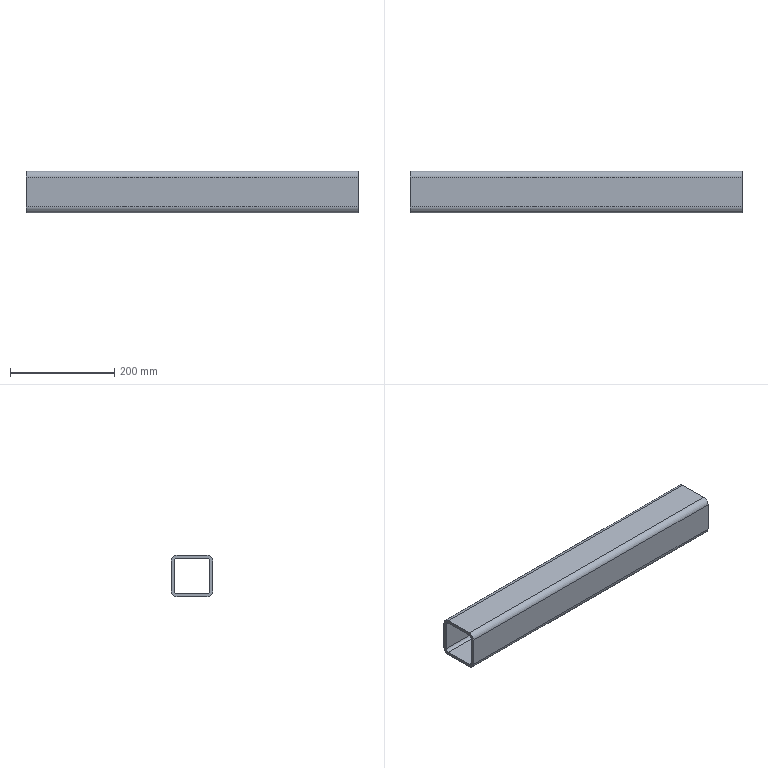Part | SolidWorks | features Extrusion 1 | 1 solid | 18 faces | box 638 x 80 x 80 mm | volume 1029649 mm3 | plane 10 | cylinder 8 | commonest cylinder face diameters 11.429 x4 22.857 x4
STEP:
#1=CARTESIAN_POINT('',(249.,-40.,-28.571));
#2=VERTEX_POINT('',#1);
#3=CARTESIAN_POINT('',(249.,-28.571,-40.));
#4=VERTEX_POINT('',#3);
#5=CARTESIAN_POINT('',(249.,-28.571,-28.571));
#6=DIRECTION('',(1.,0.,0.));
#7=DIRECTION('',(0.,0.,-1.));
#8=AXIS2_PLACEMENT_3D('',#5,#6,#7);
#9=CIRCLE('',#8,11.429);
#10=EDGE_CURVE('',#2,#4,#9,.T.);
#11=ORIENTED_EDGE('',*,*,#10,.F.);
#12=CARTESIAN_POINT('',(-389.,-40.,-28.571));
#13=VERTEX_POINT('',#12);
#14=CARTESIAN_POINT('',(-389.,-40.,-28.571));
#15=DIRECTION('',(1.,0.,0.));
#16=VECTOR('',#15,1000.);
#17=LINE('',#14,#16);
#18=EDGE_CURVE('',#13,#2,#17,.T.);
#19=ORIENTED_EDGE('',*,*,#18,.F.);
#20=CARTESIAN_POINT('',(-389.,-28.571,-40.));
#21=VERTEX_POINT('',#20);
#22=CARTESIAN_POINT('',(-389.,-28.571,-28.571));
#23=DIRECTION('',(1.,0.,0.));
#24=DIRECTION('',(0.,0.,-1.));
#25=AXIS2_PLACEMENT_3D('',#22,#23,#24);
#26=CIRCLE('',#25,11.429);
#27=EDGE_CURVE('',#13,#21,#26,.T.);
#28=ORIENTED_EDGE('',*,*,#27,.T.);
#29=CARTESIAN_POINT('',(-389.,-28.571,-40.));
#30=DIRECTION('',(1.,0.,0.));
#31=VECTOR('',#30,1000.);
#32=LINE('',#29,#31);
#33=EDGE_CURVE('',#21,#4,#32,.T.);
#34=ORIENTED_EDGE('',*,*,#33,.T.);
#35=EDGE_LOOP('',(#11,#19,#28,#34));
#36=FACE_OUTER_BOUND('',#35,.T.);
#37=CARTESIAN_POINT('',(-389.,-28.571,-28.571));
#38=DIRECTION('',(1.,0.,0.));
#39=DIRECTION('',(0.,0.,-1.));
#40=AXIS2_PLACEMENT_3D('',#37,#38,#39);
#41=CYLINDRICAL_SURFACE('',#40,11.429);
#42=ADVANCED_FACE('',(#36),#41,.T.);
#43=CARTESIAN_POINT('',(249.,-40.,28.571));
#44=VERTEX_POINT('',#43);
#45=CARTESIAN_POINT('',(249.,-40.,28.571));
#46=DIRECTION('',(0.,0.,-1.));
#47=VECTOR('',#46,1000.);
#48=LINE('',#45,#47);
#49=EDGE_CURVE('',#44,#2,#48,.T.);
#50=ORIENTED_EDGE('',*,*,#49,.F.);
#51=CARTESIAN_POINT('',(-389.,-40.,28.571));
#52=VERTEX_POINT('',#51);
#53=CARTESIAN_POINT('',(-389.,-40.,28.571));
#54=DIRECTION('',(1.,0.,0.));
#55=VECTOR('',#54,1000.);
#56=LINE('',#53,#55);
#57=EDGE_CURVE('',#52,#44,#56,.T.);
#58=ORIENTED_EDGE('',*,*,#57,.F.);
#59=CARTESIAN_POINT('',(-389.,-40.,28.571));
#60=DIRECTION('',(0.,0.,-1.));
#61=VECTOR('',#60,1000.);
#62=LINE('',#59,#61);
#63=EDGE_CURVE('',#52,#13,#62,.T.);
#64=ORIENTED_EDGE('',*,*,#63,.T.);
#65=ORIENTED_EDGE('',*,*,#18,.T.);
#66=EDGE_LOOP('',(#50,#58,#64,#65));
#67=FACE_OUTER_BOUND('',#66,.T.);
#68=CARTESIAN_POINT('',(-389.,-40.,28.571));
#69=DIRECTION('',(0.,-1.,0.));
#70=DIRECTION('',(0.,0.,-1.));
#71=AXIS2_PLACEMENT_3D('',#68,#69,#70);
#72=PLANE('',#71);
#73=ADVANCED_FACE('',(#67),#72,.T.);
#74=CARTESIAN_POINT('',(249.,-28.571,40.));
#75=VERTEX_POINT('',#74);
#76=CARTESIAN_POINT('',(249.,-28.571,28.571));
#77=DIRECTION('',(1.,0.,0.));
#78=DIRECTION('',(0.,0.,-1.));
#79=AXIS2_PLACEMENT_3D('',#76,#77,#78);
#80=CIRCLE('',#79,11.429);
#81=EDGE_CURVE('',#75,#44,#80,.T.);
#82=ORIENTED_EDGE('',*,*,#81,.F.);
#83=CARTESIAN_POINT('',(-389.,-28.571,40.));
#84=VERTEX_POINT('',#83);
#85=CARTESIAN_POINT('',(-389.,-28.571,40.));
#86=DIRECTION('',(1.,0.,0.));
#87=VECTOR('',#86,1000.);
#88=LINE('',#85,#87);
#89=EDGE_CURVE('',#84,#75,#88,.T.);
#90=ORIENTED_EDGE('',*,*,#89,.F.);
#91=CARTESIAN_POINT('',(-389.,-28.571,28.571));
#92=DIRECTION('',(1.,0.,0.));
#93=DIRECTION('',(0.,0.,-1.));
#94=AXIS2_PLACEMENT_3D('',#91,#92,#93);
#95=CIRCLE('',#94,11.429);
#96=EDGE_CURVE('',#84,#52,#95,.T.);
#97=ORIENTED_EDGE('',*,*,#96,.T.);
#98=ORIENTED_EDGE('',*,*,#57,.T.);
#99=EDGE_LOOP('',(#82,#90,#97,#98));
#100=FACE_OUTER_BOUND('',#99,.T.);
#101=CARTESIAN_POINT('',(-389.,-28.571,28.571));
#102=DIRECTION('',(1.,0.,0.));
#103=DIRECTION('',(0.,0.,-1.));
#104=AXIS2_PLACEMENT_3D('',#101,#102,#103);
#105=CYLINDRICAL_SURFACE('',#104,11.429);
#106=ADVANCED_FACE('',(#100),#105,.T.);
#107=CARTESIAN_POINT('',(249.,28.571,40.));
#108=VERTEX_POINT('',#107);
#109=CARTESIAN_POINT('',(249.,28.571,40.));
#110=DIRECTION('',(0.,-1.,0.));
#111=VECTOR('',#110,1000.);
#112=LINE('',#109,#111);
#113=EDGE_CURVE('',#108,#75,#112,.T.);
#114=ORIENTED_EDGE('',*,*,#113,.F.);
#115=CARTESIAN_POINT('',(-389.,28.571,40.));
#116=VERTEX_POINT('',#115);
#117=CARTESIAN_POINT('',(-389.,28.571,40.));
#118=DIRECTION('',(1.,0.,0.));
#119=VECTOR('',#118,1000.);
#120=LINE('',#117,#119);
#121=EDGE_CURVE('',#116,#108,#120,.T.);
#122=ORIENTED_EDGE('',*,*,#121,.F.);
#123=CARTESIAN_POINT('',(-389.,28.571,40.));
#124=DIRECTION('',(0.,-1.,0.));
#125=VECTOR('',#124,1000.);
#126=LINE('',#123,#125);
#127=EDGE_CURVE('',#116,#84,#126,.T.);
#128=ORIENTED_EDGE('',*,*,#127,.T.);
#129=ORIENTED_EDGE('',*,*,#89,.T.);
#130=EDGE_LOOP('',(#114,#122,#128,#129));
#131=FACE_OUTER_BOUND('',#130,.T.);
#132=CARTESIAN_POINT('',(-389.,28.571,40.));
#133=DIRECTION('',(0.,0.,1.));
#134=DIRECTION('',(1.,0.,0.));
#135=AXIS2_PLACEMENT_3D('',#132,#133,#134);
#136=PLANE('',#135);
#137=ADVANCED_FACE('',(#131),#136,.T.);
#138=CARTESIAN_POINT('',(249.,40.,28.571));
#139=VERTEX_POINT('',#138);
#140=CARTESIAN_POINT('',(249.,28.571,28.571));
#141=DIRECTION('',(1.,0.,0.));
#142=DIRECTION('',(0.,0.,-1.));
#143=AXIS2_PLACEMENT_3D('',#140,#141,#142);
#144=CIRCLE('',#143,11.429);
#145=EDGE_CURVE('',#139,#108,#144,.T.);
#146=ORIENTED_EDGE('',*,*,#145,.F.);
#147=CARTESIAN_POINT('',(-389.,40.,28.571));
#148=VERTEX_POINT('',#147);
#149=CARTESIAN_POINT('',(-389.,40.,28.571));
#150=DIRECTION('',(1.,0.,0.));
#151=VECTOR('',#150,1000.);
#152=LINE('',#149,#151);
#153=EDGE_CURVE('',#148,#139,#152,.T.);
#154=ORIENTED_EDGE('',*,*,#153,.F.);
#155=CARTESIAN_POINT('',(-389.,28.571,28.571));
#156=DIRECTION('',(1.,0.,0.));
#157=DIRECTION('',(0.,0.,-1.));
#158=AXIS2_PLACEMENT_3D('',#155,#156,#157);
#159=CIRCLE('',#158,11.429);
#160=EDGE_CURVE('',#148,#116,#159,.T.);
#161=ORIENTED_EDGE('',*,*,#160,.T.);
#162=ORIENTED_EDGE('',*,*,#121,.T.);
#163=EDGE_LOOP('',(#146,#154,#161,#162));
#164=FACE_OUTER_BOUND('',#163,.T.);
#165=CARTESIAN_POINT('',(-389.,28.571,28.571));
#166=DIRECTION('',(1.,0.,0.));
#167=DIRECTION('',(0.,0.,-1.));
#168=AXIS2_PLACEMENT_3D('',#165,#166,#167);
#169=CYLINDRICAL_SURFACE('',#168,11.429);
#170=ADVANCED_FACE('',(#164),#169,.T.);
#171=CARTESIAN_POINT('',(249.,40.,-28.571));
#172=VERTEX_POINT('',#171);
#173=CARTESIAN_POINT('',(249.,40.,-28.571));
#174=DIRECTION('',(0.,0.,1.));
#175=VECTOR('',#174,1000.);
#176=LINE('',#173,#175);
#177=EDGE_CURVE('',#172,#139,#176,.T.);
#178=ORIENTED_EDGE('',*,*,#177,.F.);
#179=CARTESIAN_POINT('',(-389.,40.,-28.571));
#180=VERTEX_POINT('',#179);
#181=CARTESIAN_POINT('',(-389.,40.,-28.571));
#182=DIRECTION('',(1.,0.,0.));
#183=VECTOR('',#182,1000.);
#184=LINE('',#181,#183);
#185=EDGE_CURVE('',#180,#172,#184,.T.);
#186=ORIENTED_EDGE('',*,*,#185,.F.);
#187=CARTESIAN_POINT('',(-389.,40.,-28.571));
#188=DIRECTION('',(0.,0.,1.));
#189=VECTOR('',#188,1000.);
#190=LINE('',#187,#189);
#191=EDGE_CURVE('',#180,#148,#190,.T.);
#192=ORIENTED_EDGE('',*,*,#191,.T.);
#193=ORIENTED_EDGE('',*,*,#153,.T.);
#194=EDGE_LOOP('',(#178,#186,#192,#193));
#195=FACE_OUTER_BOUND('',#194,.T.);
#196=CARTESIAN_POINT('',(-389.,40.,-28.571));
#197=DIRECTION('',(0.,1.,0.));
#198=DIRECTION('',(0.,0.,1.));
#199=AXIS2_PLACEMENT_3D('',#196,#197,#198);
#200=PLANE('',#199);
#201=ADVANCED_FACE('',(#195),#200,.T.);
#202=CARTESIAN_POINT('',(249.,28.571,-40.));
#203=VERTEX_POINT('',#202);
#204=CARTESIAN_POINT('',(249.,28.571,-28.571));
#205=DIRECTION('',(1.,0.,0.));
#206=DIRECTION('',(0.,0.,-1.));
#207=AXIS2_PLACEMENT_3D('',#204,#205,#206);
#208=CIRCLE('',#207,11.429);
#209=EDGE_CURVE('',#203,#172,#208,.T.);
#210=ORIENTED_EDGE('',*,*,#209,.F.);
#211=CARTESIAN_POINT('',(-389.,28.571,-40.));
#212=VERTEX_POINT('',#211);
#213=CARTESIAN_POINT('',(-389.,28.571,-40.));
#214=DIRECTION('',(1.,0.,0.));
#215=VECTOR('',#214,1000.);
#216=LINE('',#213,#215);
#217=EDGE_CURVE('',#212,#203,#216,.T.);
#218=ORIENTED_EDGE('',*,*,#217,.F.);
#219=CARTESIAN_POINT('',(-389.,28.571,-28.571));
#220=DIRECTION('',(1.,0.,0.));
#221=DIRECTION('',(0.,0.,-1.));
#222=AXIS2_PLACEMENT_3D('',#219,#220,#221);
#223=CIRCLE('',#222,11.429);
#224=EDGE_CURVE('',#212,#180,#223,.T.);
#225=ORIENTED_EDGE('',*,*,#224,.T.);
#226=ORIENTED_EDGE('',*,*,#185,.T.);
#227=EDGE_LOOP('',(#210,#218,#225,#226));
#228=FACE_OUTER_BOUND('',#227,.T.);
#229=CARTESIAN_POINT('',(-389.,28.571,-28.571));
#230=DIRECTION('',(1.,0.,0.));
#231=DIRECTION('',(0.,0.,-1.));
#232=AXIS2_PLACEMENT_3D('',#229,#230,#231);
#233=CYLINDRICAL_SURFACE('',#232,11.429);
#234=ADVANCED_FACE('',(#228),#233,.T.);
#235=CARTESIAN_POINT('',(249.,-28.571,-40.));
#236=DIRECTION('',(0.,1.,0.));
#237=VECTOR('',#236,1000.);
#238=LINE('',#235,#237);
#239=EDGE_CURVE('',#4,#203,#238,.T.);
#240=ORIENTED_EDGE('',*,*,#239,.F.);
#241=ORIENTED_EDGE('',*,*,#33,.F.);
#242=CARTESIAN_POINT('',(-389.,-28.571,-40.));
#243=DIRECTION('',(0.,1.,0.));
#244=VECTOR('',#243,1000.);
#245=LINE('',#242,#244);
#246=EDGE_CURVE('',#21,#212,#245,.T.);
#247=ORIENTED_EDGE('',*,*,#246,.T.);
#248=ORIENTED_EDGE('',*,*,#217,.T.);
#249=EDGE_LOOP('',(#240,#241,#247,#248));
#250=FACE_OUTER_BOUND('',#249,.T.);
#251=CARTESIAN_POINT('',(-389.,-28.571,-40.));
#252=DIRECTION('',(0.,0.,-1.));
#253=DIRECTION('',(-1.,0.,0.));
#254=AXIS2_PLACEMENT_3D('',#251,#252,#253);
#255=PLANE('',#254);
#256=ADVANCED_FACE('',(#250),#255,.T.);
#257=CARTESIAN_POINT('',(-389.,28.571,34.286));
#258=VERTEX_POINT('',#257);
#259=CARTESIAN_POINT('',(-389.,-28.571,34.286));
#260=VERTEX_POINT('',#259);
#261=CARTESIAN_POINT('',(-389.,-28.571,34.286));
#262=DIRECTION('',(0.,-1.,0.));
#263=VECTOR('',#262,1000.);
#264=LINE('',#261,#263);
#265=EDGE_CURVE('',#258,#260,#264,.T.);
#266=ORIENTED_EDGE('',*,*,#265,.T.);
#267=CARTESIAN_POINT('',(-389.,-34.286,28.571));
#268=VERTEX_POINT('',#267);
#269=CARTESIAN_POINT('',(-389.,-28.571,28.571));
#270=DIRECTION('',(1.,0.,0.));
#271=DIRECTION('',(0.,0.,1.));
#272=AXIS2_PLACEMENT_3D('',#269,#270,#271);
#273=CIRCLE('',#272,5.714);
#274=EDGE_CURVE('',#260,#268,#273,.T.);
#275=ORIENTED_EDGE('',*,*,#274,.T.);
#276=CARTESIAN_POINT('',(-389.,-34.286,-28.571));
#277=VERTEX_POINT('',#276);
#278=CARTESIAN_POINT('',(-389.,-34.286,-28.571));
#279=DIRECTION('',(0.,0.,-1.));
#280=VECTOR('',#279,1000.);
#281=LINE('',#278,#280);
#282=EDGE_CURVE('',#268,#277,#281,.T.);
#283=ORIENTED_EDGE('',*,*,#282,.T.);
#284=CARTESIAN_POINT('',(-389.,-28.571,-34.286));
#285=VERTEX_POINT('',#284);
#286=CARTESIAN_POINT('',(-389.,-28.571,-28.571));
#287=DIRECTION('',(1.,0.,0.));
#288=DIRECTION('',(0.,0.,1.));
#289=AXIS2_PLACEMENT_3D('',#286,#287,#288);
#290=CIRCLE('',#289,5.714);
#291=EDGE_CURVE('',#277,#285,#290,.T.);
#292=ORIENTED_EDGE('',*,*,#291,.T.);
#293=CARTESIAN_POINT('',(-389.,28.571,-34.286));
#294=VERTEX_POINT('',#293);
#295=CARTESIAN_POINT('',(-389.,28.571,-34.286));
#296=DIRECTION('',(0.,1.,0.));
#297=VECTOR('',#296,1000.);
#298=LINE('',#295,#297);
#299=EDGE_CURVE('',#285,#294,#298,.T.);
#300=ORIENTED_EDGE('',*,*,#299,.T.);
#301=CARTESIAN_POINT('',(-389.,34.286,-28.571));
#302=VERTEX_POINT('',#301);
#303=CARTESIAN_POINT('',(-389.,28.571,-28.571));
#304=DIRECTION('',(1.,0.,0.));
#305=DIRECTION('',(0.,0.,1.));
#306=AXIS2_PLACEMENT_3D('',#303,#304,#305);
#307=CIRCLE('',#306,5.714);
#308=EDGE_CURVE('',#294,#302,#307,.T.);
#309=ORIENTED_EDGE('',*,*,#308,.T.);
#310=CARTESIAN_POINT('',(-389.,34.286,28.571));
#311=VERTEX_POINT('',#310);
#312=CARTESIAN_POINT('',(-389.,34.286,28.571));
#313=DIRECTION('',(0.,0.,1.));
#314=VECTOR('',#313,1000.);
#315=LINE('',#312,#314);
#316=EDGE_CURVE('',#302,#311,#315,.T.);
#317=ORIENTED_EDGE('',*,*,#316,.T.);
#318=CARTESIAN_POINT('',(-389.,28.571,28.571));
#319=DIRECTION('',(1.,0.,0.));
#320=DIRECTION('',(0.,0.,1.));
#321=AXIS2_PLACEMENT_3D('',#318,#319,#320);
#322=CIRCLE('',#321,5.714);
#323=EDGE_CURVE('',#311,#258,#322,.T.);
#324=ORIENTED_EDGE('',*,*,#323,.T.);
#325=EDGE_LOOP('',(#266,#275,#283,#292,#300,#309,#317,#324));
#326=FACE_BOUND('',#325,.T.);
#327=ORIENTED_EDGE('',*,*,#27,.F.);
#328=ORIENTED_EDGE('',*,*,#63,.F.);
#329=ORIENTED_EDGE('',*,*,#96,.F.);
#330=ORIENTED_EDGE('',*,*,#127,.F.);
#331=ORIENTED_EDGE('',*,*,#160,.F.);
#332=ORIENTED_EDGE('',*,*,#191,.F.);
#333=ORIENTED_EDGE('',*,*,#224,.F.);
#334=ORIENTED_EDGE('',*,*,#246,.F.);
#335=EDGE_LOOP('',(#327,#328,#329,#330,#331,#332,#333,#334));
#336=FACE_OUTER_BOUND('',#335,.T.);
#337=CARTESIAN_POINT('',(-389.,-28.571,-28.571));
#338=DIRECTION('',(1.,0.,0.));
#339=DIRECTION('',(0.,0.,-1.));
#340=AXIS2_PLACEMENT_3D('',#337,#338,#339);
#341=PLANE('',#340);
#342=ADVANCED_FACE('',(#326,#336),#341,.F.);
#343=CARTESIAN_POINT('',(249.,-28.571,34.286));
#344=VERTEX_POINT('',#343);
#345=CARTESIAN_POINT('',(249.,-34.286,28.571));
#346=VERTEX_POINT('',#345);
#347=CARTESIAN_POINT('',(249.,-28.571,28.571));
#348=DIRECTION('',(1.,0.,0.));
#349=DIRECTION('',(0.,0.,1.));
#350=AXIS2_PLACEMENT_3D('',#347,#348,#349);
#351=CIRCLE('',#350,5.714);
#352=EDGE_CURVE('',#344,#346,#351,.T.);
#353=ORIENTED_EDGE('',*,*,#352,.F.);
#354=CARTESIAN_POINT('',(249.,28.571,34.286));
#355=VERTEX_POINT('',#354);
#356=CARTESIAN_POINT('',(249.,-28.571,34.286));
#357=DIRECTION('',(0.,-1.,0.));
#358=VECTOR('',#357,1000.);
#359=LINE('',#356,#358);
#360=EDGE_CURVE('',#355,#344,#359,.T.);
#361=ORIENTED_EDGE('',*,*,#360,.F.);
#362=CARTESIAN_POINT('',(249.,34.286,28.571));
#363=VERTEX_POINT('',#362);
#364=CARTESIAN_POINT('',(249.,28.571,28.571));
#365=DIRECTION('',(1.,0.,0.));
#366=DIRECTION('',(0.,0.,1.));
#367=AXIS2_PLACEMENT_3D('',#364,#365,#366);
#368=CIRCLE('',#367,5.714);
#369=EDGE_CURVE('',#363,#355,#368,.T.);
#370=ORIENTED_EDGE('',*,*,#369,.F.);
#371=CARTESIAN_POINT('',(249.,34.286,-28.571));
#372=VERTEX_POINT('',#371);
#373=CARTESIAN_POINT('',(249.,34.286,28.571));
#374=DIRECTION('',(0.,0.,1.));
#375=VECTOR('',#374,1000.);
#376=LINE('',#373,#375);
#377=EDGE_CURVE('',#372,#363,#376,.T.);
#378=ORIENTED_EDGE('',*,*,#377,.F.);
#379=CARTESIAN_POINT('',(249.,28.571,-34.286));
#380=VERTEX_POINT('',#379);
#381=CARTESIAN_POINT('',(249.,28.571,-28.571));
#382=DIRECTION('',(1.,0.,0.));
#383=DIRECTION('',(0.,0.,1.));
#384=AXIS2_PLACEMENT_3D('',#381,#382,#383);
#385=CIRCLE('',#384,5.714);
#386=EDGE_CURVE('',#380,#372,#385,.T.);
#387=ORIENTED_EDGE('',*,*,#386,.F.);
#388=CARTESIAN_POINT('',(249.,-28.571,-34.286));
#389=VERTEX_POINT('',#388);
#390=CARTESIAN_POINT('',(249.,28.571,-34.286));
#391=DIRECTION('',(0.,1.,0.));
#392=VECTOR('',#391,1000.);
#393=LINE('',#390,#392);
#394=EDGE_CURVE('',#389,#380,#393,.T.);
#395=ORIENTED_EDGE('',*,*,#394,.F.);
#396=CARTESIAN_POINT('',(249.,-34.286,-28.571));
#397=VERTEX_POINT('',#396);
#398=CARTESIAN_POINT('',(249.,-28.571,-28.571));
#399=DIRECTION('',(1.,0.,0.));
#400=DIRECTION('',(0.,0.,1.));
#401=AXIS2_PLACEMENT_3D('',#398,#399,#400);
#402=CIRCLE('',#401,5.714);
#403=EDGE_CURVE('',#397,#389,#402,.T.);
#404=ORIENTED_EDGE('',*,*,#403,.F.);
#405=CARTESIAN_POINT('',(249.,-34.286,-28.571));
#406=DIRECTION('',(0.,0.,-1.));
#407=VECTOR('',#406,1000.);
#408=LINE('',#405,#407);
#409=EDGE_CURVE('',#346,#397,#408,.T.);
#410=ORIENTED_EDGE('',*,*,#409,.F.);
#411=EDGE_LOOP('',(#353,#361,#370,#378,#387,#395,#404,#410));
#412=FACE_BOUND('',#411,.T.);
#413=ORIENTED_EDGE('',*,*,#10,.T.);
#414=ORIENTED_EDGE('',*,*,#239,.T.);
#415=ORIENTED_EDGE('',*,*,#209,.T.);
#416=ORIENTED_EDGE('',*,*,#177,.T.);
#417=ORIENTED_EDGE('',*,*,#145,.T.);
#418=ORIENTED_EDGE('',*,*,#113,.T.);
#419=ORIENTED_EDGE('',*,*,#81,.T.);
#420=ORIENTED_EDGE('',*,*,#49,.T.);
#421=EDGE_LOOP('',(#413,#414,#415,#416,#417,#418,#419,#420));
#422=FACE_OUTER_BOUND('',#421,.T.);
#423=CARTESIAN_POINT('',(249.,-28.571,-28.571));
#424=DIRECTION('',(1.,0.,0.));
#425=DIRECTION('',(0.,0.,-1.));
#426=AXIS2_PLACEMENT_3D('',#423,#424,#425);
#427=PLANE('',#426);
#428=ADVANCED_FACE('',(#412,#422),#427,.T.);
#429=ORIENTED_EDGE('',*,*,#352,.T.);
#430=CARTESIAN_POINT('',(-389.,-34.286,28.571));
#431=DIRECTION('',(1.,0.,0.));
#432=VECTOR('',#431,1000.);
#433=LINE('',#430,#432);
#434=EDGE_CURVE('',#268,#346,#433,.T.);
#435=ORIENTED_EDGE('',*,*,#434,.F.);
#436=ORIENTED_EDGE('',*,*,#274,.F.);
#437=CARTESIAN_POINT('',(-389.,-28.571,34.286));
#438=DIRECTION('',(1.,0.,0.));
#439=VECTOR('',#438,1000.);
#440=LINE('',#437,#439);
#441=EDGE_CURVE('',#260,#344,#440,.T.);
#442=ORIENTED_EDGE('',*,*,#441,.T.);
#443=EDGE_LOOP('',(#429,#435,#436,#442));
#444=FACE_OUTER_BOUND('',#443,.T.);
#445=CARTESIAN_POINT('',(-389.,-28.571,28.571));
#446=DIRECTION('',(1.,0.,0.));
#447=DIRECTION('',(0.,0.,-1.));
#448=AXIS2_PLACEMENT_3D('',#445,#446,#447);
#449=CYLINDRICAL_SURFACE('',#448,5.714);
#450=ADVANCED_FACE('',(#444),#449,.F.);
#451=ORIENTED_EDGE('',*,*,#360,.T.);
#452=ORIENTED_EDGE('',*,*,#441,.F.);
#453=ORIENTED_EDGE('',*,*,#265,.F.);
#454=CARTESIAN_POINT('',(-389.,28.571,34.286));
#455=DIRECTION('',(1.,0.,0.));
#456=VECTOR('',#455,1000.);
#457=LINE('',#454,#456);
#458=EDGE_CURVE('',#258,#355,#457,.T.);
#459=ORIENTED_EDGE('',*,*,#458,.T.);
#460=EDGE_LOOP('',(#451,#452,#453,#459));
#461=FACE_OUTER_BOUND('',#460,.T.);
#462=CARTESIAN_POINT('',(-389.,-28.571,34.286));
#463=DIRECTION('',(0.,0.,1.));
#464=DIRECTION('',(1.,0.,0.));
#465=AXIS2_PLACEMENT_3D('',#462,#463,#464);
#466=PLANE('',#465);
#467=ADVANCED_FACE('',(#461),#466,.F.);
#468=ORIENTED_EDGE('',*,*,#369,.T.);
#469=ORIENTED_EDGE('',*,*,#458,.F.);
#470=ORIENTED_EDGE('',*,*,#323,.F.);
#471=CARTESIAN_POINT('',(-389.,34.286,28.571));
#472=DIRECTION('',(1.,0.,0.));
#473=VECTOR('',#472,1000.);
#474=LINE('',#471,#473);
#475=EDGE_CURVE('',#311,#363,#474,.T.);
#476=ORIENTED_EDGE('',*,*,#475,.T.);
#477=EDGE_LOOP('',(#468,#469,#470,#476));
#478=FACE_OUTER_BOUND('',#477,.T.);
#479=CARTESIAN_POINT('',(-389.,28.571,28.571));
#480=DIRECTION('',(1.,0.,0.));
#481=DIRECTION('',(0.,0.,-1.));
#482=AXIS2_PLACEMENT_3D('',#479,#480,#481);
#483=CYLINDRICAL_SURFACE('',#482,5.714);
#484=ADVANCED_FACE('',(#478),#483,.F.);
#485=ORIENTED_EDGE('',*,*,#377,.T.);
#486=ORIENTED_EDGE('',*,*,#475,.F.);
#487=ORIENTED_EDGE('',*,*,#316,.F.);
#488=CARTESIAN_POINT('',(-389.,34.286,-28.571));
#489=DIRECTION('',(1.,0.,0.));
#490=VECTOR('',#489,1000.);
#491=LINE('',#488,#490);
#492=EDGE_CURVE('',#302,#372,#491,.T.);
#493=ORIENTED_EDGE('',*,*,#492,.T.);
#494=EDGE_LOOP('',(#485,#486,#487,#493));
#495=FACE_OUTER_BOUND('',#494,.T.);
#496=CARTESIAN_POINT('',(-389.,34.286,28.571));
#497=DIRECTION('',(0.,1.,0.));
#498=DIRECTION('',(0.,0.,1.));
#499=AXIS2_PLACEMENT_3D('',#496,#497,#498);
#500=PLANE('',#499);
#501=ADVANCED_FACE('',(#495),#500,.F.);
#502=ORIENTED_EDGE('',*,*,#386,.T.);
#503=ORIENTED_EDGE('',*,*,#492,.F.);
#504=ORIENTED_EDGE('',*,*,#308,.F.);
#505=CARTESIAN_POINT('',(-389.,28.571,-34.286));
#506=DIRECTION('',(1.,0.,0.));
#507=VECTOR('',#506,1000.);
#508=LINE('',#505,#507);
#509=EDGE_CURVE('',#294,#380,#508,.T.);
#510=ORIENTED_EDGE('',*,*,#509,.T.);
#511=EDGE_LOOP('',(#502,#503,#504,#510));
#512=FACE_OUTER_BOUND('',#511,.T.);
#513=CARTESIAN_POINT('',(-389.,28.571,-28.571));
#514=DIRECTION('',(1.,0.,0.));
#515=DIRECTION('',(0.,0.,-1.));
#516=AXIS2_PLACEMENT_3D('',#513,#514,#515);
#517=CYLINDRICAL_SURFACE('',#516,5.714);
#518=ADVANCED_FACE('',(#512),#517,.F.);
#519=ORIENTED_EDGE('',*,*,#394,.T.);
#520=ORIENTED_EDGE('',*,*,#509,.F.);
#521=ORIENTED_EDGE('',*,*,#299,.F.);
#522=CARTESIAN_POINT('',(-389.,-28.571,-34.286));
#523=DIRECTION('',(1.,0.,0.));
#524=VECTOR('',#523,1000.);
#525=LINE('',#522,#524);
#526=EDGE_CURVE('',#285,#389,#525,.T.);
#527=ORIENTED_EDGE('',*,*,#526,.T.);
#528=EDGE_LOOP('',(#519,#520,#521,#527));
#529=FACE_OUTER_BOUND('',#528,.T.);
#530=CARTESIAN_POINT('',(-389.,28.571,-34.286));
#531=DIRECTION('',(0.,0.,-1.));
#532=DIRECTION('',(-1.,0.,0.));
#533=AXIS2_PLACEMENT_3D('',#530,#531,#532);
#534=PLANE('',#533);
#535=ADVANCED_FACE('',(#529),#534,.F.);
#536=ORIENTED_EDGE('',*,*,#403,.T.);
#537=ORIENTED_EDGE('',*,*,#526,.F.);
#538=ORIENTED_EDGE('',*,*,#291,.F.);
#539=CARTESIAN_POINT('',(-389.,-34.286,-28.571));
#540=DIRECTION('',(1.,0.,0.));
#541=VECTOR('',#540,1000.);
#542=LINE('',#539,#541);
#543=EDGE_CURVE('',#277,#397,#542,.T.);
#544=ORIENTED_EDGE('',*,*,#543,.T.);
#545=EDGE_LOOP('',(#536,#537,#538,#544));
#546=FACE_OUTER_BOUND('',#545,.T.);
#547=CARTESIAN_POINT('',(-389.,-28.571,-28.571));
#548=DIRECTION('',(1.,0.,0.));
#549=DIRECTION('',(0.,0.,-1.));
#550=AXIS2_PLACEMENT_3D('',#547,#548,#549);
#551=CYLINDRICAL_SURFACE('',#550,5.714);
#552=ADVANCED_FACE('',(#546),#551,.F.);
#553=ORIENTED_EDGE('',*,*,#409,.T.);
#554=ORIENTED_EDGE('',*,*,#543,.F.);
#555=ORIENTED_EDGE('',*,*,#282,.F.);
#556=ORIENTED_EDGE('',*,*,#434,.T.);
#557=EDGE_LOOP('',(#553,#554,#555,#556));
#558=FACE_OUTER_BOUND('',#557,.T.);
#559=CARTESIAN_POINT('',(-389.,-34.286,-28.571));
#560=DIRECTION('',(0.,-1.,0.));
#561=DIRECTION('',(0.,0.,-1.));
#562=AXIS2_PLACEMENT_3D('',#559,#560,#561);
#563=PLANE('',#562);
#564=ADVANCED_FACE('',(#558),#563,.F.);
#565=CLOSED_SHELL('',(#42,#73,#106,#137,#170,#201,#234,#256,#342,#428,#450,#467,#484,#501,#518,#535,#552,#564));
#566=MANIFOLD_SOLID_BREP('',#565);
#567=CARTESIAN_POINT('',(0.,0.,0.));
#568=DIRECTION('',(0.,0.,1.));
#569=DIRECTION('',(1.,0.,0.));
#570=AXIS2_PLACEMENT_3D('',#567,#568,#569);
#571=(LENGTH_UNIT()NAMED_UNIT(*)SI_UNIT(.MILLI.,.METRE.));
#572=UNCERTAINTY_MEASURE_WITH_UNIT(LENGTH_MEASURE(0.00001),#571,'','');
#573=(NAMED_UNIT(*)PLANE_ANGLE_UNIT()SI_UNIT($,.RADIAN.));
#574=(NAMED_UNIT(*)SI_UNIT($,.STERADIAN.)SOLID_ANGLE_UNIT());
#575=(GEOMETRIC_REPRESENTATION_CONTEXT(3)GLOBAL_UNCERTAINTY_ASSIGNED_CONTEXT((#572))GLOBAL_UNIT_ASSIGNED_CONTEXT((#571,#573,#574))REPRESENTATION_CONTEXT('',''));
#576=ADVANCED_BREP_SHAPE_REPRESENTATION('',(#566,#570),#575);